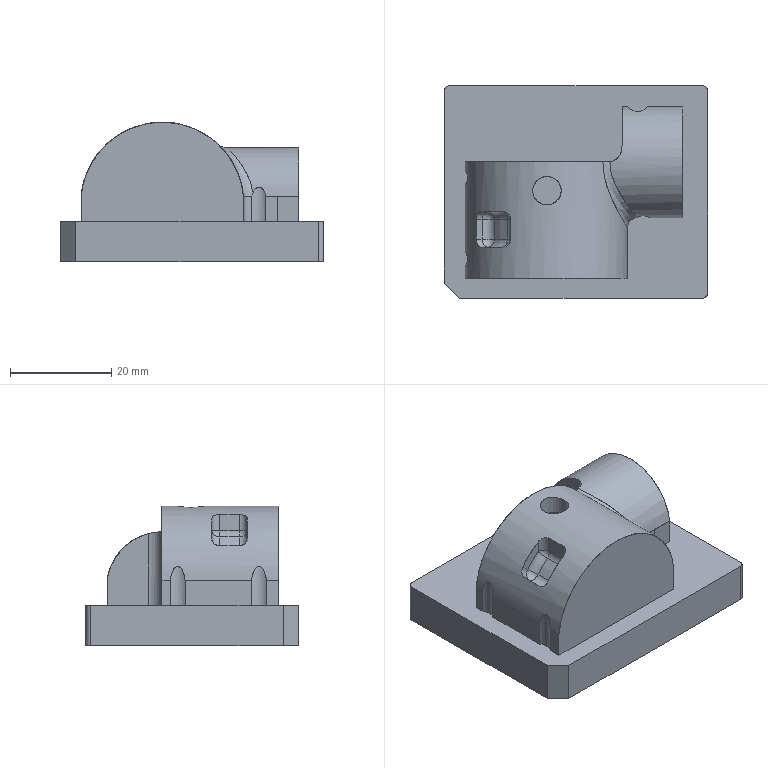NC program | PowerMill | posted with a generic post | part box 52 x 42 x 27.622 mm
Lines 1 to 929 of 214543:
%
O0001
N104 ( POWERMILL CB  : 2026004.0)
N105 ( POST VER      : 2026.0.0.5161)
N106 ( OPTION FILE   : FANUC)
N107 ( OUTPUT WORKPLANE : WORLD)
N108 (  )
N109 ( TOOL LIST )
N110 (---------------------------------------)
N111 ( NO. | ID        | DIA.| TIP RAD|LENGTH)
N112 (---------------------------------------)
N113 (    1|D10C_2_1_1 |10.0 |  0.0   |83.08 )
N114 (    2|D4C_2_1    | 4.0 |  0.0   |74.68 )
N115 (   28|D2C_2_1    | 2.0 |  0.0   | 64.8 )
N116 (    3|D10_1_1_1  |10.0 |  0.0   | 82.8 )
N117 (    7|R2_2_1     | 4.0 |  2.0   | 71.6 )
N118 (   10|D3_2_1     | 3.0 |  0.0   |74.76 )
N119 (    4|R1_1_1     | 2.0 |  1.0   |64.72 )
N120 (   13|TEXT_D4_1_1| 4.0 |  0.3   |74.88 )
N121 (---------------------------------------)
N122 (  )
N123 ( NUMBER OF TOOLPATHS: 13.0 )
N124 ( ESTIMATED PROGRAM DURATION: 0 HOURS 27 MIN 1 SEC)
N125 (  )
N126 G00 G21 G80 G40 G17
N127 G90
N128 G54
N129 G53 Z0.0
N130 (---------------)
N131 ( START TOOLPATH : 粗公开粗01-扫面平行-D10C )
N132 (---------------)
N133 ( TOOL NO.    :1 )
N134 ( TOOL TYPE   : ENDMILL)
N135 ( TOOL ID     : D10C_2_1_1)
N136 ( TOOL DIA    : 10.0 LENGTH 83.08)
N137 T1
N138 M6
N139 S8000 M03
N140 G00 G90 X0.0 Y0.0
N141 G43 Z10.2 H1
N142
N143 G05 P10000 R4
N144 X33.65 Y23.65
N145 Z1.002
N146 G01 Z-0.198 F6000.0
N147 X28.65 F10000.0
N148 X-28.65
N149 Y17.7375
N150 X28.65
N151 Y11.825
N152 X-28.65
N153 Y5.9125
N154 X28.65
N155 Y0.0
N156 X-28.65
N157 Y-5.9125
N158 X28.65
N159 Y-11.825
N160 X-28.65
N161 Y-17.7375
N162 X28.65
N163 Y-23.65
N164 X-28.65
N165 X-33.65
N166 G00 Z10.2
N167 G05 P0
N168 (---------------)
N169 ( END TOOLPATH : 粗公开粗01-扫面平行-D10C )
N170 (---------------)
N171 ( START TOOLPATH : 粗公开粗01-外形偏置-D10C )
N172 (---------------)
N173 G00 X-0.4155 Y-0.186 Z9.8022
N174 G05 P10000 R4
N175 X2.3984 Y-30.085
N176 Z0.5556
N177 G01 Z-0.6444 F6000.0
N178 Y-29.5575 F10000.0
N179 G03 X-2.3491 Y-24.81 I-4.7475 J0.0
N180 G01 X-28.579
N181 G02 X-29.579 Y-23.81 I0.0 J1.0
N182 G01 Y23.438
N183 G02 X-28.579 Y24.438 I1.0 J0.0
N184 G01 X27.748
N185 G02 X28.748 Y23.438 I0.0 J-1.0
N186 G01 Y-23.81
N187 G02 X27.748 Y-24.81 I-1.0 J0.0
N188 G01 X-2.3491
N189 Y-22.3112
N190 X-9.3099
N191 X-10.0833 Y-22.265
N192 X-10.8568 Y-22.101
N193 X-11.6302 Y-21.8041
N194 X-12.4036 Y-21.3461
N195 X-13.177 Y-20.6646
N196 X-13.7614 Y-19.9084
N197 X-13.9505 Y-19.581
N198 X-14.1615 Y-19.1349
N199 X-14.4124 Y-18.3615
N200 X-14.5375 Y-17.5881
N201 X-14.5673 Y-12.9475
N202 X-14.5401 Y-12.1741
N203 Y-10.6273
N204 X-14.5813 Y-9.0804
N205 X-14.5403 Y-0.5727
N206 X-14.578 Y0.2007
N207 X-14.5441 Y6.3881
N208 X-14.4148 Y7.1616
N209 X-14.1587 Y7.935
N210 X-13.9505 Y8.3836
N211 X-13.7549 Y8.7084
N212 X-13.177 Y9.4525
N213 X-12.4036 Y10.1326
N214 X-12.2273 Y10.2553
N215 X-11.6302 Y10.5922
N216 X-10.8568 Y10.8859
N217 X-10.211 Y11.0287
N218 X-9.3099 Y11.0914
N219 X-2.3491
N220 X-1.5554 Y11.0287
N221 X-0.8022 Y10.8492
N222 X-0.0288 Y10.5336
N223 X0.4564 Y10.2553
N224 X0.7446 Y10.0493
N225 X1.3834 Y9.4818
N226 X1.9869 Y8.7084
N227 X2.3918 Y7.935
N228 X2.6465 Y7.1616
N229 X2.7739 Y6.3881
N230 X2.7742 Y5.9245
N231 X8.8032 Y7.2046
N232 X14.2121 Y8.3531
N233 X14.2837 Y8.0159
N234 G02 X14.6791 Y3.9199 I-17.852 J-3.7905
N235 G01 X14.4182 Y-11.6623
N236 G03 X15.5417 Y-12.8285 I1.147 J-0.0192
N237 G01 X16.0873 Y-12.8397
N238 G03 X17.2579 Y-11.6937 I0.0235 J1.147
N239 G01 X17.2781 Y11.0861
N240 G03 X15.2874 Y12.8811 I-1.8032 J0.0015
N241 G03 X13.711 Y10.7131 I0.1875 J-1.7935
N242 G01 X14.2121 Y8.3531
N243 X8.8032 Y7.2046
N244 G03 X-1.9815 Y16.962 I-12.5345 J-3.0154
N245 G01 X-5.3276 Y17.4204
N246 G03 X-20.942 Y3.2446 I-1.8673 J-13.6305
N247 G01 X-20.1375 Y-17.0359
N248 G02 X-21.5736 Y-18.8162 I-1.7362 J-0.0688
N249 G01 X-21.934 Y-18.8794
N250 G02 X-23.9717 Y-17.1533 I-0.3002 J1.7115
N251 G01 X-23.6881 Y16.564
N252 G02 X-21.6882 Y18.5472 I1.9999 J-0.0168
N253 G01 X20.8572
N254 G02 X22.8572 Y16.5472 I0.0 J-2.0
N255 G01 Y-16.9192
N256 G02 X20.8778 Y-18.9191 I-2.0 J0.0
N257 G01 X10.7445 Y-19.0236
N258 G02 X8.7243 Y-16.9822 I-0.0207 J1.9999
N259 G01 X9.1581 Y3.9217
N260 G03 X8.8032 Y7.2046 I-12.8895 J0.2675
N261 G01 X2.7742 Y5.9245
N262 X2.7749 Y4.8413
N263 X2.8108 Y0.2007
N264 X2.7667 Y-0.5727
N265 X2.7662 Y-12.1741
N266 X2.7669 Y-12.1871
N267 X2.8064 Y-12.9475
N268 X2.7799 Y-17.5881
N269 X2.6584 Y-18.3615
N270 X2.4065 Y-19.1349
N271 X2.004 Y-19.9084
N272 X1.4074 Y-20.6818
N273 X0.7446 Y-21.2759
N274 X0.4939 Y-21.4552
N275 X-0.0288 Y-21.7562
N276 X-0.8022 Y-22.0712
N277 X-1.4319 Y-22.2287
N278 X-2.3491 Y-22.3112
N279 Y-24.81
N280 G00 Z3.2093
N281 G01 X2.3984 Y-30.085
N282 G00 Z0.1593
N283 G01 Z-1.0407 F6000.0
N284 Y-29.5575 F10000.0
N285 G03 X-2.3491 Y-24.81 I-4.7475 J0.0
N286 G01 X-28.579
N287 G02 X-29.579 Y-23.81 I0.0 J1.0
N288 G01 Y23.438
N289 G02 X-28.579 Y24.438 I1.0 J0.0
N290 G01 X27.748
N291 G02 X28.748 Y23.438 I0.0 J-1.0
N292 G01 Y-0.3101
N293 X22.8572 Y-0.3025
N294 X16.9204 Y-0.2948
N295 X16.9364 Y12.0791
N296 G03 X16.3898 Y12.6264 I-0.5466 J0.0007
N297 G01 X15.1196 Y12.6266
N298 G03 X14.8072 Y12.1466 I0.0 J-0.3416
N299 G01 X14.9675 Y11.7848
N300 G02 X16.5675 Y3.787 I-17.1273 J-7.5855
N301 G01 X16.2057 Y-12.6467
N302 G03 X16.532 Y-12.9874 I0.3334 J-0.0073
N303 G01 X16.5775 Y-12.9884
N304 G03 X16.9044 Y-12.6686 I0.0067 J0.3202
N305 G01 X16.9204 Y-0.2948
N306 X22.8572 Y-0.3025
N307 Y-16.9192
N308 G02 X20.8819 Y-18.919 I-2.0 J0.0
N309 G01 X12.207 Y-19.026
N310 G02 X10.1828 Y-16.9815 I-0.0247 J1.9998
N311 G01 X10.6502 Y3.906
N312 G03 X-1.7457 Y17.0263 I-12.8376 J0.2872
N313 G01 X-8.6684 Y17.2646
N314 G03 X-22.3809 Y3.4719 I-0.4564 J-13.259
N315 G01 X-21.5309 Y-17.6451
N316 G02 X-22.3911 Y-18.6012 I-0.9202 J-0.037
N317 G01 X-23.0418 Y-18.6437
N318 G02 X-24.0541 Y-17.6851 I-0.0619 J0.9484
N319 G01 X-23.6881 Y16.5686
N320 G02 X-21.6882 Y18.5472 I1.9999 J-0.0214
N321 G01 X20.8572
N322 G02 X22.8572 Y16.5472 I0.0 J-2.0
N323 G01 Y-0.3025
N324 X28.748 Y-0.3101
N325 Y-23.81
N326 G02 X27.748 Y-24.81 I-1.0 J0.0
N327 G01 X-0.8019
N328 X-0.8022 Y-22.3101
N329 X-2.3394 Y-22.3102
N330 X-2.3491 Y-22.3111
N331 X-9.3099
N332 X-9.3119 Y-22.311
N333 X-10.8568 Y-22.3112
N334 X-11.6302 Y-22.2531
N335 X-12.4036 Y-22.0732
N336 X-13.177 Y-21.7592
N337 X-13.7031 Y-21.4552
N338 X-13.9505 Y-21.2776
N339 X-14.6183 Y-20.6818
N340 X-15.2146 Y-19.9084
N341 X-15.6159 Y-19.1349
N342 X-15.869 Y-18.3615
N343 X-15.9914 Y-17.5881
N344 X-15.9895 Y-16.0412
N345 X-16.0136 Y-12.9475
N346 X-16.0146 Y2.521
N347 X-16.002 Y6.3881
N348 X-15.8737 Y7.1616
N349 X-15.6199 Y7.935
N350 X-15.2124 Y8.7084
N351 X-14.7239 Y9.3569
N352 X-13.9505 Y10.0674
N353 X-13.6839 Y10.2553
N354 X-13.177 Y10.5457
N355 X-12.4036 Y10.8581
N356 X-11.6728 Y11.0287
N357 X-10.8568 Y11.0914
N358 X-9.3132 Y11.0911
N359 X-9.3099 Y11.0913
N360 X-2.3491
N361 X-2.3304 Y11.0898
N362 X-0.8022 Y11.0896
N363 X-0.0908 Y11.0287
N364 X0.7446 Y10.8223
N365 X1.5181 Y10.4891
N366 X1.9168 Y10.2553
N367 X2.2915 Y9.9862
N368 X2.8436 Y9.4818
N369 X3.0649 Y9.231
N370 X3.4474 Y8.7084
N371 X3.8512 Y7.935
N372 X4.1078 Y7.1616
N373 X4.235 Y6.3881
N374 X4.2628 Y0.2007
N375 X4.2321 Y-0.5727
N376 Y-0.5826
N377 Y-12.1741
N378 X4.2486 Y-12.9475
N379 X4.2358 Y-17.5881
N380 X4.1104 Y-18.3615
N381 X3.8585 Y-19.1349
N382 X3.4596 Y-19.9084
N383 X3.0649 Y-20.4483
N384 X2.8611 Y-20.6818
N385 X2.2915 Y-21.2058
N386 X1.9468 Y-21.4552
N387 X1.5181 Y-21.7083
N388 X0.7446 Y-22.0417
N389 X0.0219 Y-22.2287
N390 X-0.8022 Y-22.3101
N391 X-0.8019 Y-24.81
N392 X-2.3491
N393 G00 Z2.8129
N394 G01 X2.3984 Y-30.085
N395 G00 Z-0.2371
N396 G01 Z-1.4371 F6000.0
N397 Y-29.5575 F10000.0
N398 G03 X-2.3491 Y-24.81 I-4.7475 J0.0
N399 G01 X-28.579
N400 G02 X-29.579 Y-23.81 I0.0 J1.0
N401 G01 Y23.438
N402 G02 X-28.579 Y24.438 I1.0 J0.0
N403 G01 X27.748
N404 G02 X28.748 Y23.438 I0.0 J-1.0
N405 G01 Y-0.4823
N406 X22.9337 Y-0.4709
N407 X17.5773 Y-0.4604
N408 X17.602 Y12.1286
N409 G03 X16.4418 Y13.292 I-1.1611 J0.0023
N410 G01 X16.0685 Y13.2923
N411 G03 X15.3929 Y12.2992 I-0.0006 J-0.7259
N412 G01 X15.6546 Y11.6382
N413 G02 X16.8266 Y5.2692 I-15.5452 J-6.1529
N414 G01 X16.5899 Y-13.0405
N415 G03 X16.9796 Y-13.4392 I0.3936 J-0.0051
N416 G01 X17.1564 Y-13.441
N417 G03 X17.5527 Y-13.0494 I0.0039 J0.3923
N418 G01 X17.5773 Y-0.4604
N419 X22.9337 Y-0.4709
N420 Y-17.7149
N421 G02 X21.6529 Y-18.9957 I-1.2808 J0.0
N422 G01 X12.2557
N423 G02 X11.1374 Y-17.8598 I0.0 J1.1184
N424 G01 X11.4994 Y5.293
N425 G03 X7.7263 Y13.968 I-11.4478 J0.179
N426 G01 X7.4508 Y14.2169
N427 G03 X-0.0903 Y17.1247 I-7.5571 J-8.3659
N428 G01 X-11.4611 Y17.1409
N429 G03 X-19.828 Y13.5607 I-0.0164 J-11.5284
N430 G01 X-19.927 Y13.4566
N431 G03 X-23.0427 Y5.5907 I8.1875 J-7.793
N432 G01 X-22.8881 Y-17.8277
N433 X-22.8269 Y-18.3453
N434 G02 X-23.1383 Y-18.7171 I-0.3285 J-0.0411
N435 G01 X-23.4064 Y-18.7309
N436 G02 X-23.7545 Y-18.4004 I-0.017 J0.3306
N437 G01 X-23.7647 Y17.3425
N438 G02 X-22.4839 Y18.6237 I1.2808 J0.0004
N439 G01 X21.6529
N440 G02 X22.9337 Y17.3429 I0.0 J-1.2808
N441 G01 Y-0.4709
N442 X28.748 Y-0.4823
N443 Y-23.81
N444 G02 X27.748 Y-24.81 I-1.0 J0.0
N445 G01 X0.1632
N446 X0.0679 Y-22.3075
N447 X-0.0288 Y-22.3112
N448 X-11.6302
N449 X-12.4036 Y-22.291
N450 X-13.177 Y-22.1629
N451 X-13.9505 Y-21.9075
N452 X-14.7239 Y-21.4997
N453 X-15.4973 Y-20.8946
N454 X-15.7083 Y-20.6818
N455 X-16.2707 Y-19.9624
N456 X-16.7061 Y-19.1349
N457 X-16.9586 Y-18.3615
N458 X-17.0826 Y-17.5881
N459 X-17.0803 Y-12.1741
N460 X-17.1015 Y-9.0804
N461 X-17.0951 Y3.2944
N462 X-17.0708 Y6.3881
N463 X-16.9434 Y7.1616
N464 X-16.688 Y7.935
N465 X-16.2841 Y8.7084
N466 X-15.6799 Y9.4818
N467 X-15.4973 Y9.6613
N468 X-14.7531 Y10.2553
N469 X-13.9505 Y10.6814
N470 X-13.177 Y10.9399
N471 X-12.7412 Y11.0287
N472 X-12.4036 Y11.0702
N473 X-11.6302 Y11.0914
N474 X-0.0288
N475 X0.7446 Y11.0608
N476 X1.5181 Y10.9158
N477 X2.2915 Y10.6397
N478 X3.003 Y10.2553
N479 X3.8383 Y9.5697
N480 X4.5323 Y8.7084
N481 X4.9347 Y7.935
N482 X5.19 Y7.1616
N483 X5.3205 Y6.3881
N484 X5.3462 Y0.2007
N485 X5.3152 Y-0.5727
N486 Y-0.5827
N487 Y-12.1741
N488 X5.3373 Y-12.9475
N489 X5.3263 Y-17.5881
N490 X5.2013 Y-18.3615
N491 X4.9502 Y-19.1349
N492 X4.6118 Y-19.807
N493 X3.9527 Y-20.6818
N494 X3.8383 Y-20.7996
N495 X3.0649 Y-21.4365
N496 X2.2915 Y-21.8661
N497 X1.5181 Y-22.1387
N498 X1.1129 Y-22.2287
N499 X0.7446 Y-22.2817
N500 X0.0679 Y-22.3075
N501 X0.1632 Y-24.81
N502 X-2.3491
N503 G00 Z2.4165
N504 G01 X2.3984 Y-30.085
N505 G00 Z-0.6335
N506 G01 Z-1.8335 F6000.0
N507 Y-29.5575 F10000.0
N508 G03 X-2.3491 Y-24.81 I-4.7475 J0.0
N509 G01 X-28.579
N510 G02 X-29.579 Y-23.81 I0.0 J1.0
N511 G01 Y23.438
N512 G02 X-28.579 Y24.438 I1.0 J0.0
N513 G01 X27.748
N514 G02 X28.748 Y23.438 I0.0 J-1.0
N515 G01 Y-0.2425
N516 X23.033
N517 X17.5643
N518 Y13.0388
N519 G03 X17.3488 Y13.2543 I-0.2155 J0.0
N520 G01 X15.9423
N521 G03 X15.8209 Y13.0634 I0.0 J-0.134
N522 G01 X15.9034 Y12.8871
N523 G02 X17.3622 Y7.3189 I-14.3982 J-6.7471
N524 G01 X17.3736 Y7.1599
N525 X17.4139 Y6.0536
N526 X17.4174 Y3.7629
N527 X17.421 Y-3.5906
N528 X17.4117 Y-10.9441
N529 X17.4061 Y-13.5237
N530 X17.4223 Y-13.5631
N531 X17.4617 Y-13.5795
N532 X17.5085
N533 X17.5479 Y-13.5633
N534 X17.5643 Y-13.5238
N535 Y-0.2425
N536 X23.033
N537 Y-18.8533
N538 G02 X22.7913 Y-19.095 I-0.2417 J0.0
N539 G01 X11.9967 Y-19.0951
N540 G02 X11.7984 Y-18.8572 I0.0 J0.2017
N541 G01 X11.8168 Y-18.7561
N542 X11.9033 Y-18.1223
N543 X11.9328 Y-17.4834
N544 X11.9527 Y0.0437
N545 X11.9457 Y6.0482
N546 X11.9405 Y6.3582
N547 X11.9256 Y6.6678
N548 X11.9171 Y6.8008
N549 G03 X8.8491 Y13.5529 I-10.4276 J-0.6651
N550 G01 X8.648 Y13.7524
N551 G03 X1.2605 Y16.8291 I-7.4697 J-7.5281
N552 G01 X1.0713 Y16.8306
N553 X-12.4153 Y16.866
N554 X-12.8482 Y16.8592
N555 X-13.2804 Y16.8368
N556 X-13.4176 Y16.8272
N557 G03 X-18.1717 Y15.3968 I0.7861 J-11.2278
N558 G01 X-18.2576 Y15.3482
N559 G03 X-20.1009 Y14.0149 I5.0293 J-8.8939
N560 G01 X-20.2318 Y13.8952
N561 X-20.4456 Y13.6904
N562 X-20.7618 Y13.3662
N563 X-21.0598 Y13.0252
N564 X-21.3393 Y12.6873
N565 G03 X-22.2186 Y11.3972 I6.4938 J-5.3707
N566 G01 X-22.3901 Y11.0873
N567 G03 X-23.1194 Y9.4207 I8.5714 J-4.7438
N568 G01 X-23.1645 Y9.2843
N569 G03 X-23.5411 Y7.7529 I9.5569 J-3.1619
N570 G01 X-23.559 Y7.6436
N571 G03 X-23.6891 Y6.0577 I9.7151 J-1.5947
N572 G01 X-23.7032 Y-9.8327
N573 X-23.6882 Y-17.4974
N574 X-23.6614 Y-18.0934
N575 X-23.5835 Y-18.6848
N576 X-23.5464 Y-18.8958
N577 X-23.5563 Y-18.9792
N578 X-23.6104 Y-19.0433
N579 X-23.6261 Y-19.0535
N580 G02 X-23.8598 Y-18.9268 I-0.0825 J0.1267
N581 G01 X-23.864 Y18.4813
N582 G02 X-23.6223 Y18.723 I0.2417 J0.0
N583 G01 X22.7913
N584 G02 X23.033 Y18.4813 I0.0 J-0.2417
N585 G01 Y-0.2425
N586 X28.748
N587 Y-23.81
N588 G02 X27.748 Y-24.81 I-1.0 J0.0
N589 G01 X1.5795
N590 X1.5181 Y-22.2923
N591 X0.7446 Y-22.3112
N592 X-12.4036
N593 X-13.177 Y-22.2993
N594 X-13.9505 Y-22.1889
N595 X-14.7239 Y-21.9527
N596 X-15.4973 Y-21.5709
N597 X-15.6801 Y-21.4552
N598 X-16.2707 Y-20.9982
N599 X-16.5959 Y-20.6818
N600 X-17.0442 Y-20.13
N601 X-17.1933 Y-19.9084
N602 X-17.594 Y-19.1349
N603 X-17.8176 Y-18.4685
N604 X-17.9695 Y-17.5881
N605 X-17.9691 Y-12.1741
N606 X-17.9889 Y-9.8538
N607 X-17.988 Y-3.6664
N608 X-17.9608 Y6.3881
N609 X-17.8338 Y7.1616
N610 X-17.5779 Y7.935
N611 X-17.1738 Y8.7084
N612 X-17.0442 Y8.8995
N613 X-16.5706 Y9.4818
N614 X-16.2707 Y9.773
N615 X-15.6429 Y10.2553
N616 X-14.7239 Y10.7301
N617 X-13.9505 Y10.9673
N618 X-13.6319 Y11.0287
N619 X-13.177 Y11.0787
N620 X-12.4036 Y11.0914
N621 X0.7446
N622 X1.5181 Y11.073
N623 X1.8886 Y11.0287
N624 X2.2915 Y10.9476
N625 X3.0649 Y10.6942
N626 X3.8383 Y10.2934
N627 X4.6118 Y9.6947
N628 X4.8263 Y9.4818
N629 X5.3852 Y8.7743
N630 X5.8351 Y7.935
N631 X6.089 Y7.1616
N632 X6.2166 Y6.3881
N633 X6.2156 Y4.8413
N634 X6.2411 Y0.2007
N635 X6.2161 Y-0.5727
N636 Y-0.5808
N637 X6.2139 Y-17.5881
N638 X6.0898 Y-18.3615
N639 X5.8384 Y-19.1349
N640 X5.4377 Y-19.9084
N641 X4.8403 Y-20.6818
N642 X4.6118 Y-20.9108
N643 X3.9247 Y-21.4552
N644 X3.0649 Y-21.9127
N645 X2.2915 Y-22.1665
N646 X2.0 Y-22.2287
N647 X1.5181 Y-22.2923
N648 X1.5795 Y-24.81
N649 X-2.3491
N650 G00 Z2.0202
N651 G01 X2.3984 Y-30.085
N652 G00 Z-1.0298
N653 G01 Z-2.2298 F6000.0
N654 Y-29.5575 F10000.0
N655 G03 X-2.3491 Y-24.81 I-4.7475 J0.0
N656 G01 X-5.8295
N657 Y-22.3112
N658 X-13.177
N659 X-13.9505 Y-22.2989
N660 X-14.5217 Y-22.2287
N661 X-15.4973 Y-21.9501
N662 X-16.2707 Y-21.5657
N663 X-16.4456 Y-21.4552
N664 X-17.0442 Y-20.9916
N665 X-17.3618 Y-20.6818
N666 X-17.8176 Y-20.1204
N667 X-17.9594 Y-19.9084
N668 X-18.3601 Y-19.1349
N669 X-18.591 Y-18.4375
N670 X-18.7356 Y-17.5881
N671 X-18.772 Y-10.6273
N672 X-18.708 Y-9.8538
N673 X-18.527 Y-9.0804
N674 X-18.21 Y-8.307
N675 X-18.0593 Y-7.5336
N676 Y-6.9082
N677 X-18.0718 Y-6.7972
N678 X-18.1086 Y-6.6917
N679 X-18.4472 Y-5.9867
N680 X-18.6656 Y-5.2133
N681 X-18.764 Y-4.4398
N682 X-18.7432 Y6.3881
N683 X-18.6159 Y7.1616
N684 X-18.3611 Y7.935
N685 X-17.9561 Y8.7084
N686 X-17.8176 Y8.9137
N687 X-17.3526 Y9.4818
N688 X-17.0442 Y9.7809
N689 X-16.4255 Y10.2553
N690 X-15.4973 Y10.7322
N691 X-14.7239 Y10.9686
N692 X-14.4137 Y11.0287
N693 X-13.9505 Y11.0792
N694 X-13.177 Y11.0914
N695 X1.5181
N696 X2.2915 Y11.0731
N697 X2.6631 Y11.0287
N698 X3.0649 Y10.9485
N699 X3.8383 Y10.6959
N700 X4.6118 Y10.2949
N701 X5.3852 Y9.6955
N702 X5.6019 Y9.4818
N703 X6.1586 Y8.7772
N704 X6.6104 Y7.935
N705 X6.8653 Y7.1616
N706 X6.9925 Y6.3881
N707 X7.0003 Y3.2944
N708 X7.0148 Y0.2007
N709 X7.0133 Y-12.9475
N710 X6.9921 Y-13.721
N711 X6.9798 Y-17.5881
N712 X6.8557 Y-18.3615
N713 X6.6036 Y-19.1349
N714 X6.2037 Y-19.9084
N715 X5.6062 Y-20.6818
N716 X5.3852 Y-20.9025
N717 X4.6907 Y-21.4552
N718 X3.8383 Y-21.9108
N719 X3.0649 Y-22.1643
N720 X2.7655 Y-22.2287
N721 X2.2915 Y-22.2916
N722 X1.5181 Y-22.3112
N723 X-5.8295
N724 Y-24.81
N725 X-28.579
N726 G02 X-29.579 Y-23.81 I0.0 J1.0
N727 G01 Y23.438
N728 G02 X-28.579 Y24.438 I1.0 J0.0
N729 G01 X27.748
N730 G02 X28.748 Y23.438 I0.0 J-1.0
N731 G01 Y-0.4581
N732 X23.6174 Y-0.4558
N733 X18.2609 Y-0.4535
N734 X18.2668 Y12.9255
N735 G03 X17.2364 Y13.9568 I-1.0308 J0.0005
N736 G01 X16.3427 Y13.9571
N737 G03 X15.7893 Y13.0836 I-0.0002 J-0.612
N738 G01 X16.0552 Y12.5211
N739 G02 X17.5794 Y5.6606 I-14.3643 J-6.7908
N740 G01 X17.4939 Y-13.8306
N741 G03 X17.7691 Y-14.1077 I0.2759 J-0.0012
N742 G01 X17.9784 Y-14.1082
N743 G03 X18.2549 Y-13.8325 I0.0007 J0.2759
N744 G01 X18.2609 Y-0.4535
N745 X23.6174 Y-0.4558
N746 Y-18.8559
N747 G02 X22.7939 Y-19.6794 I-0.8235 J0.0
N748 G01 X12.6306
N749 G02 X11.964 Y-18.8749 I0.0 J0.6784
N750 G01 X11.999 Y-18.6899
N751 X12.0828 Y-18.101
N752 X12.1129 Y-17.5069
N753 X12.2329 Y5.6642
N754 G03 X1.6458 Y16.3032 I-10.584 J0.0548
N755 G01 X-13.4483 Y16.2988
N756 G03 X-23.9357 Y6.0413 I0.0031 J-10.4931
N757 G01 X-24.1043 Y-1.468
N758 G03 X-23.9544 Y-4.5745 I22.017 J-0.4945
N759 G01 X-23.6442 Y-7.1719
N760 X-23.6301 Y-7.4052
N761 X-23.6433 Y-7.6385
N762 X-23.9502 Y-10.2974
N763 G03 X-24.0603 Y-14.8085 I24.7904 J-2.8617
N764 G01 X-23.8584 Y-17.8555
N765 X-23.8043 Y-18.4046
N766 X-23.715 Y-18.949
N767 X-23.6746 Y-19.1541
N768 G02 X-23.9279 Y-19.5255 I-0.3095 J-0.061
N769 G01 X-24.0552 Y-19.5486
N770 G02 X-24.4372 Y-19.2298 I-0.0578 J0.3189
N771 G01 X-24.4484 Y18.4837
N772 G02 X-23.6249 Y19.3074 I0.8235 J0.0002
N773 G01 X22.7939
N774 G02 X23.6174 Y18.4839 I0.0 J-0.8235
N775 G01 Y-0.4558
N776 X28.748 Y-0.4581
N777 Y-23.81
N778 G02 X27.748 Y-24.81 I-1.0 J0.0
N779 G01 X-2.3491
N780 G00 Z1.6238
N781 G01 X2.3984 Y-30.085
N782 G00 Z-1.4262
N783 G01 Z-2.6262 F6000.0
N784 Y-29.5575 F10000.0
N785 G03 X-2.3491 Y-24.81 I-4.7475 J0.0
N786 G01 X-5.8295
N787 Y-22.3112
N788 X-13.9505
N789 X-14.7239 Y-22.2934
N790 X-15.4973 Y-22.1701
N791 X-16.2707 Y-21.9209
N792 X-17.0442 Y-21.5211
N793 X-17.8176 Y-20.926
N794 X-18.0616 Y-20.6818
N795 X-18.591 Y-20.0146
N796 X-19.061 Y-19.1349
N797 X-19.3123 Y-18.3615
N798 X-19.4354 Y-17.5881
N799 X-19.4542 Y-16.8147
N800 X-19.4456 Y-10.6273
N801 X-19.3644 Y-9.952
N802 X-19.1222 Y-9.0804
N803 X-18.7545 Y-8.307
N804 X-18.591 Y-8.0484
N805 X-18.338 Y-7.7244
N806 G03 X-18.3359 Y-7.1116 I-0.3941 J0.3077
N807 G01 X-18.6065 Y-6.7601
N808 X-19.0269 Y-5.9867
N809 X-19.2916 Y-5.2133
N810 X-19.427 Y-4.4398
N811 X-19.4499 Y-3.6664
N812 X-19.4272 Y6.3881
N813 X-19.3 Y7.1616
N814 X-19.0451 Y7.935
N815 X-18.6402 Y8.7084
N816 X-18.0367 Y9.4818
N817 X-17.8176 Y9.698
N818 X-17.1097 Y10.2553
N819 X-16.2707 Y10.6976
N820 X-15.4973 Y10.9487
N821 X-15.0979 Y11.0287
N822 X-14.7239 Y11.0732
N823 X-13.9505 Y11.0914
N824 X2.2915
N825 X3.0649 Y11.0647
N826 X3.8383 Y10.9273
N827 X4.6118 Y10.6602
N828 X5.3618 Y10.2553
N829 X6.1586 Y9.6142
N830 X6.2886 Y9.4818
N831 X6.8921 Y8.7084
N832 X7.297 Y7.935
N833 X7.552 Y7.1616
N834 X7.6795 Y6.3881
N835 X7.6999 Y0.2007
N836 X7.6751 Y-0.5727
N837 Y-12.1741
N838 X7.6987 Y-13.721
N839 X7.6809 Y-17.5881
N840 X7.5568 Y-18.3615
N841 X7.3053 Y-19.1349
N842 X6.9321 Y-19.8638
N843 X6.3074 Y-20.6818
N844 X6.1586 Y-20.8336
N845 X5.3852 Y-21.4584
N846 X4.6118 Y-21.8798
N847 X3.8383 Y-22.1463
N848 X3.4671 Y-22.2287
N849 X3.0649 Y-22.285
N850 X2.2915 Y-22.3112
N851 X-5.8295
N852 Y-24.81
N853 X-28.579
N854 G02 X-29.579 Y-23.81 I0.0 J1.0
N855 G01 Y23.438
N856 G02 X-28.579 Y24.438 I1.0 J0.0
N857 G01 X16.3107
N858 X16.6515 Y19.4865
N859 X16.9691 Y14.8729
N860 G03 X15.6506 Y12.7649 I0.1055 J-1.5323
N861 G01 X16.1832 Y11.4476
N862 G02 X17.2358 Y6.4796 I-13.4894 J-5.4537
N863 G01 X17.2475 Y6.1026
N864 X17.3146 Y-13.672
N865 G03 X18.1078 Y-14.4625 I0.7932 J0.0027
N866 G01 X18.3952
N867 G03 X19.1885 Y-13.6619 I0.0 J0.7932
N868 G01 X18.9408 Y12.7992
N869 G03 X18.591 Y13.8642 I-1.8489 J-0.0173
N870 G01 X18.3199 Y14.2397
N871 G03 X16.9691 Y14.8729 I-1.2453 J-0.8991
N872 G01 X16.6515 Y19.4865
N873 X23.4619
N874 G02 X23.7965 Y19.1519 I0.0 J-0.3346
N875 G01 Y-19.5239
N876 G02 X23.4619 Y-19.8585 I-0.3346 J0.0
N877 G01 X12.6053 Y-19.8586
N878 G02 X12.3653 Y-19.5584 I0.0 J0.2461
N879 G01 X12.3972 Y-19.4169
N880 X12.4472 Y-19.1824
N881 X12.4917 Y-18.9469
N882 X12.5151 Y-18.8145
N883 G03 X12.7155 Y-16.4896 I-12.8997 J2.2831
N884 G01 X12.6435 Y6.0954
N885 X12.613 Y6.7997
N886 X12.5263 Y7.4994
N887 X12.5007 Y7.655
N888 X12.3597 Y8.3428
N889 X12.1658 Y9.0177
N890 X12.1047 Y9.2031
N891 X11.9269 Y9.6923
N892 X11.7199 Y10.1699
N893 X11.6671 Y10.2823
N894 X11.3474 Y10.9027
N895 X10.983 Y11.498
N896 X10.8647 Y11.6762
N897 G03 X9.8435 Y12.9363 I-7.1193 J-4.7257
N898 G01 X9.6737 Y13.1093
N899 G03 X8.1733 Y14.3332 I-6.2697 J-6.1543
N900 G01 X8.0031 Y14.4432
N901 X7.4888 Y14.7528
N902 X6.9558 Y15.029
N903 X6.8578 Y15.0759
N904 X6.4066 Y15.2761
N905 X5.9448 Y15.4504
N906 X5.7559 Y15.5156
N907 X5.0832 Y15.7189
N908 X4.3966 Y15.8688
N909 X4.2767 Y15.8901
N910 G03 X2.5486 Y16.0426 I-1.7299 J-9.7343
N911 G01 X-14.3066 Y16.0456
N912 G03 X-18.9704 Y14.8917 I-0.0018 J-9.995
N913 G01 X-19.067 Y14.8408
N914 G03 X-20.7008 Y13.7481 I4.4055 J-8.3547
N915 G01 X-20.8851 Y13.5948
N916 X-21.1387 Y13.3746
N917 X-21.3827 Y13.1438
N918 X-21.4562 Y13.0714
N919 G03 X-22.5122 Y11.8166 I6.244 J-6.3271
N920 G01 X-22.6175 Y11.6651
N921 G03 X-23.4155 Y10.2816 I7.8102 J-5.4268
N922 G01 X-23.468 Y10.1698
N923 X-23.6751 Y9.6921
N924 X-23.8529 Y9.2027
N925 X-23.9142 Y9.0166
N926 X-24.108 Y8.3416
N927 X-24.2487 Y7.6537
N928 X-24.2746 Y7.4964
N929 X-24.3614 Y6.7922
N930 X-24.3909 Y6.0832
N931 X-24.4029 Y-3.9317
N932 G03 X-24.1856 Y-6.0012 I9.8533 J-0.0117
N933 G01 X-24.133 Y-6.2475
N934 X-24.0745 Y-6.4912
N935 X-24.0036 Y-6.7317
N936 X-23.9681 Y-6.842
N937 G02 X-23.9476 Y-7.871 I-1.7018 J-0.5486
N938 G01 X-23.9935 Y-8.0354
N939 G03 X-24.4641 Y-11.607 I12.347 J-3.4439
N940 G01 X-24.4085 Y-17.1884
N941 G03 X-24.201 Y-19.1627 I10.4935 J0.1046
N942 G01 X-24.1197 Y-19.5634
N943 G02 X-24.3361 Y-19.8573 I-0.2411 J-0.0491
N944 G02 X-24.6069 Y-19.6126 I-0.0247 J0.2448
N945 G01 X-24.6275 Y19.1517
N946 G02 X-24.2929 Y19.4865 I0.3346 J0.0002
N947 G01 X16.6515
N948 X16.3107 Y24.438
N949 X27.748
N950 G02 X28.748 Y23.438 I0.0 J-1.0
N951 G01 Y-23.81
N952 G02 X27.748 Y-24.81 I-1.0 J0.0
N953 G01 X-2.3491
N954 G00 Z1.2274
N955 G01 X2.3984 Y-30.085
N956 G00 Z-1.8226
N957 G01 Z-3.0226 F6000.0
N958 Y-29.5575 F10000.0
N959 G03 X-2.3491 Y-24.81 I-4.7475 J0.0
N960 G01 X-28.579
N961 G02 X-29.579 Y-23.81 I0.0 J1.0
N962 G01 Y23.438
N963 G02 X-28.579 Y24.438 I1.0 J0.0
N964 G01 X27.748
N965 G02 X28.748 Y23.438 I0.0 J-1.0
N966 G01 Y-0.3334
N967 X23.9366 Y-0.3331
N968 X19.0544 Y-0.3328
N969 X19.0554 Y13.9262
N970 G03 X18.2363 Y14.7454 I-0.8192 J0.0
N971 G01 X15.8544 Y14.7457
N972 G03 X15.4939 Y14.0684 I0.0 J-0.4346
N973 G01 X15.7677 Y13.6617
N974 G02 X18.5025 Y4.2091 I-13.3453 J-8.983
N975 G01 X17.9541 Y-14.5701
N976 G03 X18.3902 Y-15.083 I0.5025 J-0.0146
N977 G01 X18.4789 Y-15.0949
N978 G03 X19.0535 Y-14.5918 I0.0671 J0.5032
N979 G01 X19.0544 Y-0.3328
N980 X23.9366 Y-0.3331
N981 Y-17.9986
N982 G02 X21.975 Y-19.9982 I-2.0 J0.0
N983 G01 X15.008 Y-20.132
N984 G02 X12.9704 Y-18.0738 I-0.0384 J1.9997
N985 G01 X13.6264 Y4.3439
N986 G03 X2.2677 Y15.8999 I-11.2237 J0.3284
N987 G01 X-15.0109 Y15.6921
N988 G03 X-22.4356 Y12.1168 I0.1172 J-9.7403
N989 G01 X-23.1152 Y11.2854
N990 G02 X-24.9694 Y11.9842 I-0.8094 J0.6617
N991 G01 X-24.7664 Y17.6976
N992 G02 X-22.7676 Y19.6266 I1.9988 J-0.071
N993 G01 X21.9366
N994 G02 X23.9366 Y17.6266 I0.0 J-2.0
N995 G01 Y-0.3331
N996 X28.748 Y-0.3334
N997 Y-23.81
N998 G02 X27.748 Y-24.81 I-1.0 J0.0
N999 G01 X3.5017
N1000 X3.355 Y-22.2942
N1001 X3.0649 Y-22.3112
N1002 X-14.7239
N1003 X-15.4973 Y-22.2778
N1004 X-15.8363 Y-22.2287
N1005 X-16.2707 Y-22.1299
N1006 X-17.0442 Y-21.8512
N1007 X-17.7603 Y-21.4552
N1008 X-18.591 Y-20.7697
N1009 X-19.274 Y-19.9084
N1010 X-19.6747 Y-19.1349
N1011 X-19.9261 Y-18.3615
N1012 X-20.0502 Y-17.5881
N1013 X-20.0488 Y-10.6273
N1014 X-19.9447 Y-9.8538
N1015 X-19.7158 Y-9.0804
N1016 X-19.6743 Y-8.9943
N1017 X-24.3986 Y-7.6164
N1018 G02 X-24.6184 Y-7.585 I-0.1077 J0.0314
N1019 G01 Y-7.2604
N1020 G02 X-24.3941 I0.1121 J0.0
N1021 G01 Y-7.585
N1022 X-24.3952 Y-7.6009
N1023 X-24.3986 Y-7.6164
N1024 X-19.6743 Y-8.9943
N1025 X-19.3423 Y-8.307
N1026 X-18.9109 Y-7.7285